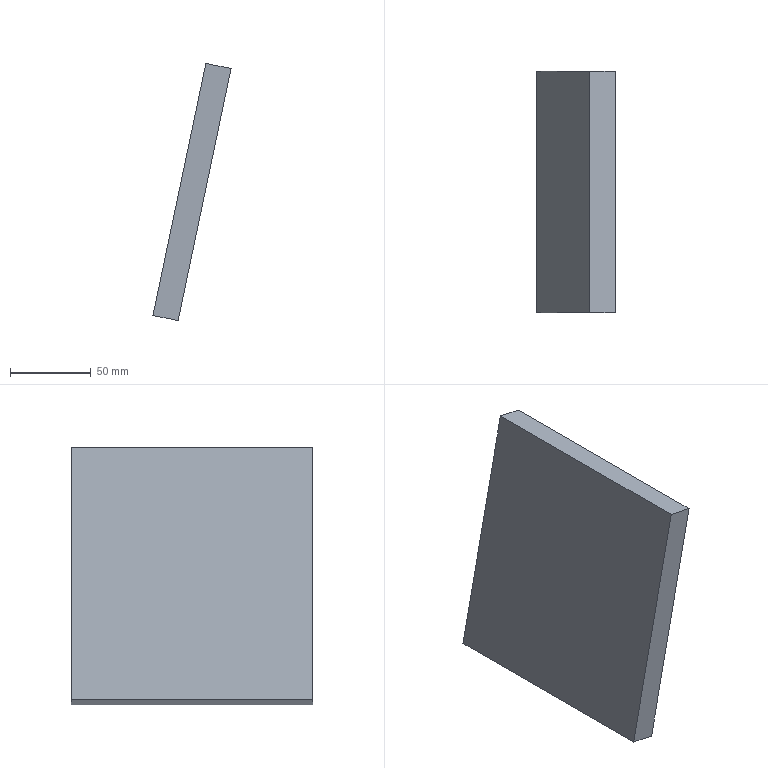Part | STEP file | 5_ESTAGIO_003-02 | 1 solid | 6 faces | box 48.561 x 150 x 159.871 mm | volume 384000 mm3 | plane 6
STEP:
#1=CARTESIAN_POINT('',(0.,0.,0.));
#2=DIRECTION('',(0.,0.,1.));
#3=DIRECTION('',(1.,0.,0.));
#4=AXIS2_PLACEMENT_3D('',#1,#2,#3);
#5=CARTESIAN_POINT('',(-2659.787,-709.15,1049.021));
#6=VERTEX_POINT('',#5);
#7=CARTESIAN_POINT('',(-2644.129,-709.15,1045.73));
#8=VERTEX_POINT('',#7);
#9=CARTESIAN_POINT('',(-2659.787,-709.15,1049.021));
#10=DIRECTION('',(0.9786,0.,-0.2056));
#11=VECTOR('',#10,1.);
#12=LINE('',#9,#11);
#13=CARTESIAN_POINT('',(98.633,0.,469.382));
#14=DIRECTION('',(-0.2056,0.,-0.9786));
#15=DIRECTION('',(-0.9786,0.,0.2056));
#16=AXIS2_PLACEMENT_3D('',#13,#14,#15);
#17=PLANE('',#16);
#18=CARTESIAN_POINT('',(2818.663,-709.15));
#19=DIRECTION('',(-1.,0.));
#20=VECTOR('',#19,1.);
#21=LINE('',#18,#20);
#22=(GEOMETRIC_REPRESENTATION_CONTEXT(2)PARAMETRIC_REPRESENTATION_CONTEXT()REPRESENTATION_CONTEXT('',''));
#23=DEFINITIONAL_REPRESENTATION('',(#21),#22);
#24=PCURVE('',#17,#23);
#25=CARTESIAN_POINT('',(-2659.787,-709.15,1049.021));
#26=DIRECTION('',(0.,1.,0.));
#27=DIRECTION('',(0.,0.,1.));
#28=AXIS2_PLACEMENT_3D('',#25,#26,#27);
#29=PLANE('',#28);
#30=CARTESIAN_POINT('',(-0.000000003,0.));
#31=DIRECTION('',(-0.2056,0.9786));
#32=VECTOR('',#31,1.);
#33=LINE('',#30,#32);
#34=(GEOMETRIC_REPRESENTATION_CONTEXT(2)PARAMETRIC_REPRESENTATION_CONTEXT()REPRESENTATION_CONTEXT('',''));
#35=DEFINITIONAL_REPRESENTATION('',(#33),#34);
#36=PCURVE('',#29,#35);
#37=SURFACE_CURVE('',#12,(#24,#36),.PCURVE_S1.);
#38=EDGE_CURVE('',#6,#8,#37,.T.);
#39=ORIENTED_EDGE('',*,*,#38,.F.);
#40=CARTESIAN_POINT('',(-2659.787,-859.15,1049.021));
#41=VERTEX_POINT('',#40);
#42=CARTESIAN_POINT('',(-2659.787,-709.15,1049.021));
#43=DIRECTION('',(0.,-1.,0.));
#44=VECTOR('',#43,1.);
#45=LINE('',#42,#44);
#46=CARTESIAN_POINT('',(2818.663,-709.15));
#47=DIRECTION('',(0.,-1.));
#48=VECTOR('',#47,1.);
#49=LINE('',#46,#48);
#50=(GEOMETRIC_REPRESENTATION_CONTEXT(2)PARAMETRIC_REPRESENTATION_CONTEXT()REPRESENTATION_CONTEXT('',''));
#51=DEFINITIONAL_REPRESENTATION('',(#49),#50);
#52=PCURVE('',#17,#51);
#53=CARTESIAN_POINT('',(-2659.787,-709.15,1049.021));
#54=DIRECTION('',(0.9786,0.,-0.2056));
#55=DIRECTION('',(-0.2056,0.,-0.9786));
#56=AXIS2_PLACEMENT_3D('',#53,#54,#55);
#57=PLANE('',#56);
#58=CARTESIAN_POINT('',(0.,0.));
#59=DIRECTION('',(0.,-1.));
#60=VECTOR('',#59,1.);
#61=LINE('',#58,#60);
#62=(GEOMETRIC_REPRESENTATION_CONTEXT(2)PARAMETRIC_REPRESENTATION_CONTEXT()REPRESENTATION_CONTEXT('',''));
#63=DEFINITIONAL_REPRESENTATION('',(#61),#62);
#64=PCURVE('',#57,#63);
#65=SURFACE_CURVE('',#45,(#52,#64),.PCURVE_S1.);
#66=EDGE_CURVE('',#6,#41,#65,.T.);
#67=ORIENTED_EDGE('',*,*,#66,.T.);
#68=CARTESIAN_POINT('',(-2644.129,-859.15,1045.73));
#69=VERTEX_POINT('',#68);
#70=CARTESIAN_POINT('',(-2644.129,-859.15,1045.73));
#71=DIRECTION('',(-0.9786,0.,0.2056));
#72=VECTOR('',#71,1.);
#73=LINE('',#70,#72);
#74=CARTESIAN_POINT('',(2802.663,-859.15));
#75=DIRECTION('',(1.,0.));
#76=VECTOR('',#75,1.);
#77=LINE('',#74,#76);
#78=(GEOMETRIC_REPRESENTATION_CONTEXT(2)PARAMETRIC_REPRESENTATION_CONTEXT()REPRESENTATION_CONTEXT('',''));
#79=DEFINITIONAL_REPRESENTATION('',(#77),#78);
#80=PCURVE('',#17,#79);
#81=CARTESIAN_POINT('',(-2644.129,-859.15,1045.73));
#82=DIRECTION('',(0.,-1.,0.));
#83=DIRECTION('',(0.,0.,-1.));
#84=AXIS2_PLACEMENT_3D('',#81,#82,#83);
#85=PLANE('',#84);
#86=CARTESIAN_POINT('',(-0.000000003,0.));
#87=DIRECTION('',(-0.2056,-0.9786));
#88=VECTOR('',#87,1.);
#89=LINE('',#86,#88);
#90=(GEOMETRIC_REPRESENTATION_CONTEXT(2)PARAMETRIC_REPRESENTATION_CONTEXT()REPRESENTATION_CONTEXT('',''));
#91=DEFINITIONAL_REPRESENTATION('',(#89),#90);
#92=PCURVE('',#85,#91);
#93=SURFACE_CURVE('',#73,(#80,#92),.PCURVE_S1.);
#94=EDGE_CURVE('',#69,#41,#93,.T.);
#95=ORIENTED_EDGE('',*,*,#94,.F.);
#96=CARTESIAN_POINT('',(-2644.129,-859.15,1045.73));
#97=DIRECTION('',(0.,1.,0.));
#98=VECTOR('',#97,1.);
#99=LINE('',#96,#98);
#100=CARTESIAN_POINT('',(2802.663,-859.15));
#101=DIRECTION('',(0.,1.));
#102=VECTOR('',#101,1.);
#103=LINE('',#100,#102);
#104=(GEOMETRIC_REPRESENTATION_CONTEXT(2)PARAMETRIC_REPRESENTATION_CONTEXT()REPRESENTATION_CONTEXT('',''));
#105=DEFINITIONAL_REPRESENTATION('',(#103),#104);
#106=PCURVE('',#17,#105);
#107=CARTESIAN_POINT('',(-2644.129,-859.15,1045.73));
#108=DIRECTION('',(-0.9786,0.,0.2056));
#109=DIRECTION('',(0.2056,0.,0.9786));
#110=AXIS2_PLACEMENT_3D('',#107,#108,#109);
#111=PLANE('',#110);
#112=CARTESIAN_POINT('',(0.,0.));
#113=DIRECTION('',(0.,1.));
#114=VECTOR('',#113,1.);
#115=LINE('',#112,#114);
#116=(GEOMETRIC_REPRESENTATION_CONTEXT(2)PARAMETRIC_REPRESENTATION_CONTEXT()REPRESENTATION_CONTEXT('',''));
#117=DEFINITIONAL_REPRESENTATION('',(#115),#116);
#118=PCURVE('',#111,#117);
#119=SURFACE_CURVE('',#99,(#106,#118),.PCURVE_S1.);
#120=EDGE_CURVE('',#69,#8,#119,.T.);
#121=ORIENTED_EDGE('',*,*,#120,.T.);
#122=EDGE_LOOP('',(#39,#67,#95,#121));
#123=FACE_BOUND('',#122,.T.);
#124=ADVANCED_FACE('',(#123),#17,.F.);
#125=CARTESIAN_POINT('',(-2692.69,-709.15,892.44));
#126=VERTEX_POINT('',#125);
#127=CARTESIAN_POINT('',(-2677.032,-709.15,889.15));
#128=VERTEX_POINT('',#127);
#129=CARTESIAN_POINT('',(-2692.69,-709.15,892.44));
#130=DIRECTION('',(0.9786,0.,-0.2056));
#131=VECTOR('',#130,1.);
#132=LINE('',#129,#131);
#133=CARTESIAN_POINT('',(-2745.535,-689.15,903.545));
#134=DIRECTION('',(-0.2056,0.,-0.9786));
#135=DIRECTION('',(-0.9786,0.,0.2056));
#136=AXIS2_PLACEMENT_3D('',#133,#134,#135);
#137=PLANE('',#136);
#138=CARTESIAN_POINT('',(-54.,-20.));
#139=DIRECTION('',(-1.,0.));
#140=VECTOR('',#139,1.);
#141=LINE('',#138,#140);
#142=(GEOMETRIC_REPRESENTATION_CONTEXT(2)PARAMETRIC_REPRESENTATION_CONTEXT()REPRESENTATION_CONTEXT('',''));
#143=DEFINITIONAL_REPRESENTATION('',(#141),#142);
#144=PCURVE('',#137,#143);
#145=CARTESIAN_POINT('',(-156.58,-32.903));
#146=DIRECTION('',(-0.2056,0.9786));
#147=VECTOR('',#146,1.);
#148=LINE('',#145,#147);
#149=(GEOMETRIC_REPRESENTATION_CONTEXT(2)PARAMETRIC_REPRESENTATION_CONTEXT()REPRESENTATION_CONTEXT('',''));
#150=DEFINITIONAL_REPRESENTATION('',(#148),#149);
#151=PCURVE('',#29,#150);
#152=SURFACE_CURVE('',#132,(#144,#151),.PCURVE_S1.);
#153=EDGE_CURVE('',#126,#128,#152,.T.);
#154=ORIENTED_EDGE('',*,*,#153,.T.);
#155=CARTESIAN_POINT('',(-2677.032,-859.15,889.15));
#156=VERTEX_POINT('',#155);
#157=CARTESIAN_POINT('',(-2677.032,-859.15,889.15));
#158=DIRECTION('',(0.,1.,0.));
#159=VECTOR('',#158,1.);
#160=LINE('',#157,#159);
#161=CARTESIAN_POINT('',(-70.,-170.));
#162=DIRECTION('',(0.,1.));
#163=VECTOR('',#162,1.);
#164=LINE('',#161,#163);
#165=(GEOMETRIC_REPRESENTATION_CONTEXT(2)PARAMETRIC_REPRESENTATION_CONTEXT()REPRESENTATION_CONTEXT('',''));
#166=DEFINITIONAL_REPRESENTATION('',(#164),#165);
#167=PCURVE('',#137,#166);
#168=CARTESIAN_POINT('',(-160.,0.));
#169=DIRECTION('',(0.,1.));
#170=VECTOR('',#169,1.);
#171=LINE('',#168,#170);
#172=(GEOMETRIC_REPRESENTATION_CONTEXT(2)PARAMETRIC_REPRESENTATION_CONTEXT()REPRESENTATION_CONTEXT('',''));
#173=DEFINITIONAL_REPRESENTATION('',(#171),#172);
#174=PCURVE('',#111,#173);
#175=SURFACE_CURVE('',#160,(#167,#174),.PCURVE_S1.);
#176=EDGE_CURVE('',#156,#128,#175,.T.);
#177=ORIENTED_EDGE('',*,*,#176,.F.);
#178=CARTESIAN_POINT('',(-2692.69,-859.15,892.44));
#179=VERTEX_POINT('',#178);
#180=CARTESIAN_POINT('',(-2677.032,-859.15,889.15));
#181=DIRECTION('',(-0.9786,0.,0.2056));
#182=VECTOR('',#181,1.);
#183=LINE('',#180,#182);
#184=CARTESIAN_POINT('',(-70.,-170.));
#185=DIRECTION('',(1.,0.));
#186=VECTOR('',#185,1.);
#187=LINE('',#184,#186);
#188=(GEOMETRIC_REPRESENTATION_CONTEXT(2)PARAMETRIC_REPRESENTATION_CONTEXT()REPRESENTATION_CONTEXT('',''));
#189=DEFINITIONAL_REPRESENTATION('',(#187),#188);
#190=PCURVE('',#137,#189);
#191=CARTESIAN_POINT('',(156.58,-32.903));
#192=DIRECTION('',(-0.2056,-0.9786));
#193=VECTOR('',#192,1.);
#194=LINE('',#191,#193);
#195=(GEOMETRIC_REPRESENTATION_CONTEXT(2)PARAMETRIC_REPRESENTATION_CONTEXT()REPRESENTATION_CONTEXT('',''));
#196=DEFINITIONAL_REPRESENTATION('',(#194),#195);
#197=PCURVE('',#85,#196);
#198=SURFACE_CURVE('',#183,(#190,#197),.PCURVE_S1.);
#199=EDGE_CURVE('',#156,#179,#198,.T.);
#200=ORIENTED_EDGE('',*,*,#199,.T.);
#201=CARTESIAN_POINT('',(-2692.69,-709.15,892.44));
#202=DIRECTION('',(0.,-1.,0.));
#203=VECTOR('',#202,1.);
#204=LINE('',#201,#203);
#205=CARTESIAN_POINT('',(-54.,-20.));
#206=DIRECTION('',(0.,-1.));
#207=VECTOR('',#206,1.);
#208=LINE('',#205,#207);
#209=(GEOMETRIC_REPRESENTATION_CONTEXT(2)PARAMETRIC_REPRESENTATION_CONTEXT()REPRESENTATION_CONTEXT('',''));
#210=DEFINITIONAL_REPRESENTATION('',(#208),#209);
#211=PCURVE('',#137,#210);
#212=CARTESIAN_POINT('',(160.,0.));
#213=DIRECTION('',(0.,-1.));
#214=VECTOR('',#213,1.);
#215=LINE('',#212,#214);
#216=(GEOMETRIC_REPRESENTATION_CONTEXT(2)PARAMETRIC_REPRESENTATION_CONTEXT()REPRESENTATION_CONTEXT('',''));
#217=DEFINITIONAL_REPRESENTATION('',(#215),#216);
#218=PCURVE('',#57,#217);
#219=SURFACE_CURVE('',#204,(#211,#218),.PCURVE_S1.);
#220=EDGE_CURVE('',#126,#179,#219,.T.);
#221=ORIENTED_EDGE('',*,*,#220,.F.);
#222=EDGE_LOOP('',(#154,#177,#200,#221));
#223=FACE_BOUND('',#222,.T.);
#224=ADVANCED_FACE('',(#223),#137,.T.);
#225=CARTESIAN_POINT('',(-2659.787,-709.15,1049.021));
#226=DIRECTION('',(-0.2056,0.,-0.9786));
#227=VECTOR('',#226,1.);
#228=LINE('',#225,#227);
#229=CARTESIAN_POINT('',(-0.000000002,0.));
#230=DIRECTION('',(-0.9786,-0.2056));
#231=VECTOR('',#230,1.);
#232=LINE('',#229,#231);
#233=(GEOMETRIC_REPRESENTATION_CONTEXT(2)PARAMETRIC_REPRESENTATION_CONTEXT()REPRESENTATION_CONTEXT('',''));
#234=DEFINITIONAL_REPRESENTATION('',(#232),#233);
#235=PCURVE('',#29,#234);
#236=CARTESIAN_POINT('',(0.000000002,0.));
#237=DIRECTION('',(1.,0.));
#238=VECTOR('',#237,1.);
#239=LINE('',#236,#238);
#240=(GEOMETRIC_REPRESENTATION_CONTEXT(2)PARAMETRIC_REPRESENTATION_CONTEXT()REPRESENTATION_CONTEXT('',''));
#241=DEFINITIONAL_REPRESENTATION('',(#239),#240);
#242=PCURVE('',#57,#241);
#243=SURFACE_CURVE('',#228,(#235,#242),.PCURVE_S1.);
#244=EDGE_CURVE('',#6,#126,#243,.T.);
#245=ORIENTED_EDGE('',*,*,#244,.F.);
#246=ORIENTED_EDGE('',*,*,#38,.T.);
#247=CARTESIAN_POINT('',(-2644.129,-709.15,1045.73));
#248=DIRECTION('',(-0.2056,0.,-0.9786));
#249=VECTOR('',#248,1.);
#250=LINE('',#247,#249);
#251=CARTESIAN_POINT('',(-3.29,15.658));
#252=DIRECTION('',(-0.9786,-0.2056));
#253=VECTOR('',#252,1.);
#254=LINE('',#251,#253);
#255=(GEOMETRIC_REPRESENTATION_CONTEXT(2)PARAMETRIC_REPRESENTATION_CONTEXT()REPRESENTATION_CONTEXT('',''));
#256=DEFINITIONAL_REPRESENTATION('',(#254),#255);
#257=PCURVE('',#29,#256);
#258=CARTESIAN_POINT('',(0.000000001,150.));
#259=DIRECTION('',(-1.,0.));
#260=VECTOR('',#259,1.);
#261=LINE('',#258,#260);
#262=(GEOMETRIC_REPRESENTATION_CONTEXT(2)PARAMETRIC_REPRESENTATION_CONTEXT()REPRESENTATION_CONTEXT('',''));
#263=DEFINITIONAL_REPRESENTATION('',(#261),#262);
#264=PCURVE('',#111,#263);
#265=SURFACE_CURVE('',#250,(#257,#264),.PCURVE_S1.);
#266=EDGE_CURVE('',#8,#128,#265,.T.);
#267=ORIENTED_EDGE('',*,*,#266,.T.);
#268=ORIENTED_EDGE('',*,*,#153,.F.);
#269=EDGE_LOOP('',(#245,#246,#267,#268));
#270=FACE_BOUND('',#269,.T.);
#271=ADVANCED_FACE('',(#270),#29,.T.);
#272=ORIENTED_EDGE('',*,*,#220,.T.);
#273=CARTESIAN_POINT('',(-2659.787,-859.15,1049.021));
#274=DIRECTION('',(-0.2056,0.,-0.9786));
#275=VECTOR('',#274,1.);
#276=LINE('',#273,#275);
#277=CARTESIAN_POINT('',(0.000000002,-150.));
#278=DIRECTION('',(1.,0.));
#279=VECTOR('',#278,1.);
#280=LINE('',#277,#279);
#281=(GEOMETRIC_REPRESENTATION_CONTEXT(2)PARAMETRIC_REPRESENTATION_CONTEXT()REPRESENTATION_CONTEXT('',''));
#282=DEFINITIONAL_REPRESENTATION('',(#280),#281);
#283=PCURVE('',#57,#282);
#284=CARTESIAN_POINT('',(-3.29,-15.658));
#285=DIRECTION('',(0.9786,-0.2056));
#286=VECTOR('',#285,1.);
#287=LINE('',#284,#286);
#288=(GEOMETRIC_REPRESENTATION_CONTEXT(2)PARAMETRIC_REPRESENTATION_CONTEXT()REPRESENTATION_CONTEXT('',''));
#289=DEFINITIONAL_REPRESENTATION('',(#287),#288);
#290=PCURVE('',#85,#289);
#291=SURFACE_CURVE('',#276,(#283,#290),.PCURVE_S1.);
#292=EDGE_CURVE('',#41,#179,#291,.T.);
#293=ORIENTED_EDGE('',*,*,#292,.F.);
#294=ORIENTED_EDGE('',*,*,#66,.F.);
#295=ORIENTED_EDGE('',*,*,#244,.T.);
#296=EDGE_LOOP('',(#272,#293,#294,#295));
#297=FACE_BOUND('',#296,.T.);
#298=ADVANCED_FACE('',(#297),#57,.F.);
#299=CARTESIAN_POINT('',(-2644.129,-859.15,1045.73));
#300=DIRECTION('',(-0.2056,0.,-0.9786));
#301=VECTOR('',#300,1.);
#302=LINE('',#299,#301);
#303=CARTESIAN_POINT('',(-0.000000001,-0.000000001));
#304=DIRECTION('',(0.9786,-0.2056));
#305=VECTOR('',#304,1.);
#306=LINE('',#303,#305);
#307=(GEOMETRIC_REPRESENTATION_CONTEXT(2)PARAMETRIC_REPRESENTATION_CONTEXT()REPRESENTATION_CONTEXT('',''));
#308=DEFINITIONAL_REPRESENTATION('',(#306),#307);
#309=PCURVE('',#85,#308);
#310=CARTESIAN_POINT('',(0.000000001,0.));
#311=DIRECTION('',(-1.,0.));
#312=VECTOR('',#311,1.);
#313=LINE('',#310,#312);
#314=(GEOMETRIC_REPRESENTATION_CONTEXT(2)PARAMETRIC_REPRESENTATION_CONTEXT()REPRESENTATION_CONTEXT('',''));
#315=DEFINITIONAL_REPRESENTATION('',(#313),#314);
#316=PCURVE('',#111,#315);
#317=SURFACE_CURVE('',#302,(#309,#316),.PCURVE_S1.);
#318=EDGE_CURVE('',#69,#156,#317,.T.);
#319=ORIENTED_EDGE('',*,*,#318,.F.);
#320=ORIENTED_EDGE('',*,*,#94,.T.);
#321=ORIENTED_EDGE('',*,*,#292,.T.);
#322=ORIENTED_EDGE('',*,*,#199,.F.);
#323=EDGE_LOOP('',(#319,#320,#321,#322));
#324=FACE_BOUND('',#323,.T.);
#325=ADVANCED_FACE('',(#324),#85,.T.);
#326=ORIENTED_EDGE('',*,*,#176,.T.);
#327=ORIENTED_EDGE('',*,*,#266,.F.);
#328=ORIENTED_EDGE('',*,*,#120,.F.);
#329=ORIENTED_EDGE('',*,*,#318,.T.);
#330=EDGE_LOOP('',(#326,#327,#328,#329));
#331=FACE_BOUND('',#330,.T.);
#332=ADVANCED_FACE('',(#331),#111,.F.);
#333=CLOSED_SHELL('',(#124,#224,#271,#298,#325,#332));
#334=MANIFOLD_SOLID_BREP('',#333);
#335=(LENGTH_UNIT()NAMED_UNIT(*)SI_UNIT(.MILLI.,.METRE.));
#336=UNCERTAINTY_MEASURE_WITH_UNIT(LENGTH_MEASURE(0.0000001),#335,'','');
#337=(NAMED_UNIT(*)PLANE_ANGLE_UNIT()SI_UNIT($,.RADIAN.));
#338=(NAMED_UNIT(*)SI_UNIT($,.STERADIAN.)SOLID_ANGLE_UNIT());
#339=(GEOMETRIC_REPRESENTATION_CONTEXT(3)GLOBAL_UNCERTAINTY_ASSIGNED_CONTEXT((#336))GLOBAL_UNIT_ASSIGNED_CONTEXT((#335,#337,#338))REPRESENTATION_CONTEXT('',''));
#340=ADVANCED_BREP_SHAPE_REPRESENTATION('',(#4,#334),#339);